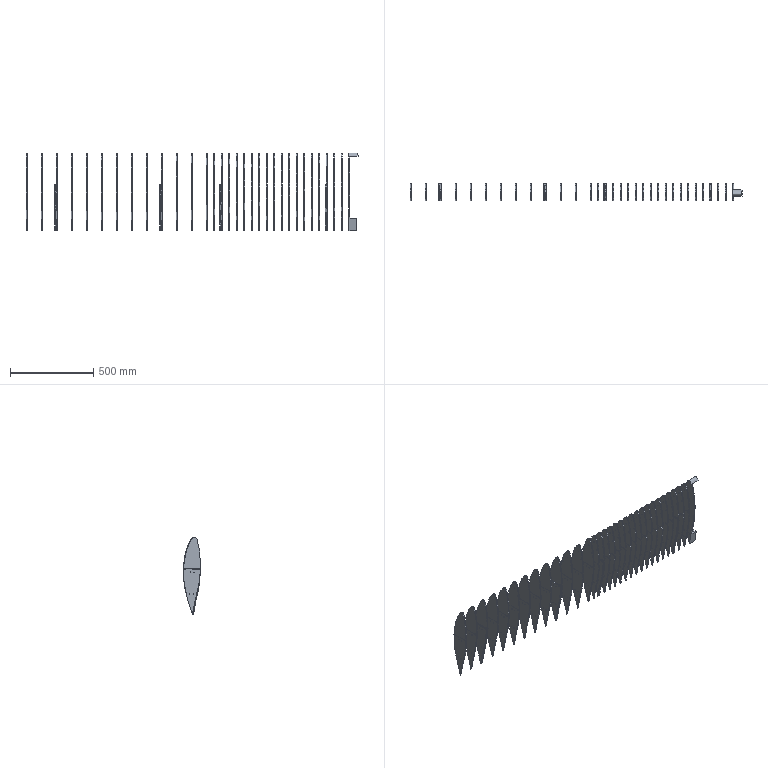Part | SolidWorks | features BaseBody 77 | 77 solids | 1373 faces | box 1989 x 103.007 x 465.475 mm | volume 6257896 mm3 | spline 632 | cylinder 412 | plane 329 | commonest cylinder face diameters 4 x412